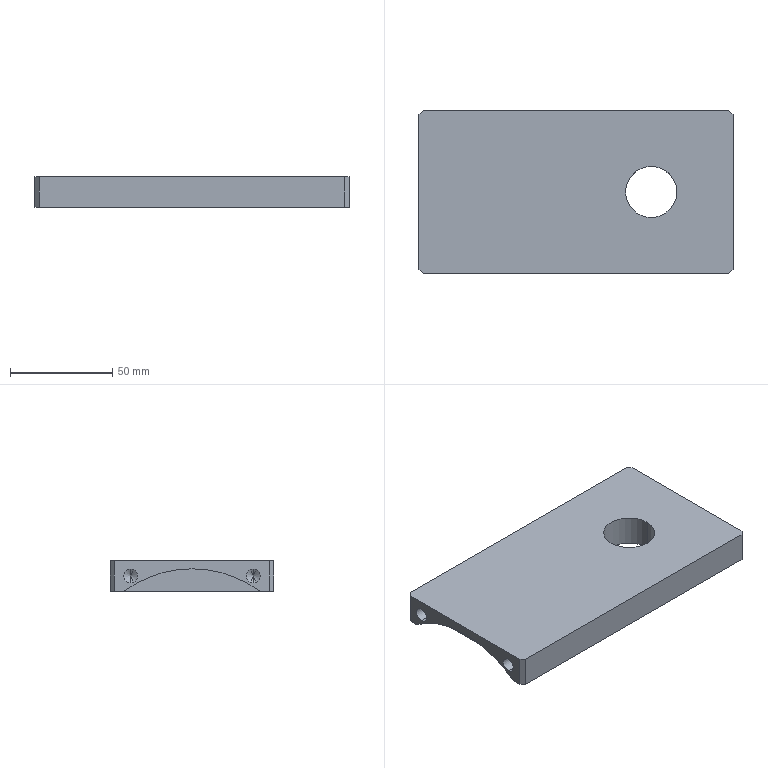Part | SolidWorks | features HoleWzd 2, Chamfer 1, Extrusion 1, ICE 1, MirrorPattern 1 | 1 solid | 31 faces | box 153.5 x 80 x 15 mm | volume 168755 mm3 | cylinder 12 | plane 11 | cone 8 | commonest cylinder face diameters 6.8 x8 25 x2 112 x2
STEP:
#1=CARTESIAN_POINT('',(-66.75,0.,3.5));
#2=VERTEX_POINT('',#1);
#3=CARTESIAN_POINT('',(-66.75,33.332,-7.5));
#4=VERTEX_POINT('',#3);
#5=CARTESIAN_POINT('',(-66.75,0.,-52.5));
#6=DIRECTION('',(-1.,0.,0.));
#7=DIRECTION('',(0.,0.,1.));
#8=AXIS2_PLACEMENT_3D('',#5,#6,#7);
#9=CIRCLE('',#8,56.);
#10=EDGE_CURVE('',#2,#4,#9,.T.);
#11=ORIENTED_EDGE('',*,*,#10,.F.);
#12=CARTESIAN_POINT('',(-76.75,0.,3.5));
#13=VERTEX_POINT('',#12);
#14=CARTESIAN_POINT('',(-66.75,0.,3.5));
#15=DIRECTION('',(-1.,0.,0.));
#16=VECTOR('',#15,1000.);
#17=LINE('',#14,#16);
#18=EDGE_CURVE('',#2,#13,#17,.T.);
#19=ORIENTED_EDGE('',*,*,#18,.T.);
#20=CARTESIAN_POINT('',(-76.75,33.332,-7.5));
#21=VERTEX_POINT('',#20);
#22=CARTESIAN_POINT('',(-76.75,0.,-52.5));
#23=DIRECTION('',(-1.,0.,0.));
#24=DIRECTION('',(0.,0.,1.));
#25=AXIS2_PLACEMENT_3D('',#22,#23,#24);
#26=CIRCLE('',#25,56.);
#27=EDGE_CURVE('',#13,#21,#26,.T.);
#28=ORIENTED_EDGE('',*,*,#27,.T.);
#29=CARTESIAN_POINT('',(-66.75,33.332,-7.5));
#30=DIRECTION('',(-1.,0.,0.));
#31=VECTOR('',#30,1000.);
#32=LINE('',#29,#31);
#33=EDGE_CURVE('',#4,#21,#32,.T.);
#34=ORIENTED_EDGE('',*,*,#33,.F.);
#35=EDGE_LOOP('',(#11,#19,#28,#34));
#36=FACE_OUTER_BOUND('',#35,.T.);
#37=CARTESIAN_POINT('',(-66.75,0.,-52.5));
#38=DIRECTION('',(-1.,0.,0.));
#39=DIRECTION('',(0.,0.,1.));
#40=AXIS2_PLACEMENT_3D('',#37,#38,#39);
#41=CYLINDRICAL_SURFACE('',#40,56.);
#42=ADVANCED_FACE('',(#36),#41,.F.);
#43=CARTESIAN_POINT('',(-57.,-30.,-3.4));
#44=VERTEX_POINT('',#43);
#45=CARTESIAN_POINT('',(-57.,-30.,3.4));
#46=VERTEX_POINT('',#45);
#47=CARTESIAN_POINT('',(-57.,-30.,0.));
#48=DIRECTION('',(-1.,0.,0.));
#49=DIRECTION('',(0.,0.,1.));
#50=AXIS2_PLACEMENT_3D('',#47,#48,#49);
#51=CIRCLE('',#50,3.4);
#52=EDGE_CURVE('',#44,#46,#51,.T.);
#53=ORIENTED_EDGE('',*,*,#52,.F.);
#54=CARTESIAN_POINT('',(-76.75,-30.,-3.4));
#55=VERTEX_POINT('',#54);
#56=CARTESIAN_POINT('',(-76.75,-30.,-3.4));
#57=DIRECTION('',(-1.,0.,0.));
#58=VECTOR('',#57,1000.);
#59=LINE('',#56,#58);
#60=EDGE_CURVE('',#44,#55,#59,.T.);
#61=ORIENTED_EDGE('',*,*,#60,.T.);
#62=CARTESIAN_POINT('',(-76.75,-30.,3.4));
#63=VERTEX_POINT('',#62);
#64=CARTESIAN_POINT('',(-76.75,-30.,0.));
#65=DIRECTION('',(-1.,0.,0.));
#66=DIRECTION('',(0.,0.,1.));
#67=AXIS2_PLACEMENT_3D('',#64,#65,#66);
#68=CIRCLE('',#67,3.4);
#69=EDGE_CURVE('',#55,#63,#68,.T.);
#70=ORIENTED_EDGE('',*,*,#69,.T.);
#71=CARTESIAN_POINT('',(-76.75,-30.,3.4));
#72=DIRECTION('',(-1.,0.,0.));
#73=VECTOR('',#72,1000.);
#74=LINE('',#71,#73);
#75=EDGE_CURVE('',#46,#63,#74,.T.);
#76=ORIENTED_EDGE('',*,*,#75,.F.);
#77=EDGE_LOOP('',(#53,#61,#70,#76));
#78=FACE_OUTER_BOUND('',#77,.T.);
#79=CARTESIAN_POINT('',(-76.75,-30.,0.));
#80=DIRECTION('',(-1.,0.,0.));
#81=DIRECTION('',(0.,0.,1.));
#82=AXIS2_PLACEMENT_3D('',#79,#80,#81);
#83=CYLINDRICAL_SURFACE('',#82,3.4);
#84=ADVANCED_FACE('',(#78),#83,.F.);
#85=CARTESIAN_POINT('',(-54.957,-30.,0.));
#86=VERTEX_POINT('',#85);
#87=CARTESIAN_POINT('',(-57.,-30.,3.4));
#88=DIRECTION('',(-0.515,0.,0.8572));
#89=VECTOR('',#88,1000.);
#90=LINE('',#87,#89);
#91=EDGE_CURVE('',#86,#46,#90,.T.);
#92=ORIENTED_EDGE('',*,*,#91,.F.);
#93=CARTESIAN_POINT('',(-57.,-30.,-3.4));
#94=DIRECTION('',(-0.515,0.,-0.8572));
#95=VECTOR('',#94,1000.);
#96=LINE('',#93,#95);
#97=EDGE_CURVE('',#86,#44,#96,.T.);
#98=ORIENTED_EDGE('',*,*,#97,.T.);
#99=ORIENTED_EDGE('',*,*,#52,.T.);
#100=EDGE_LOOP('',(#92,#98,#99));
#101=FACE_OUTER_BOUND('',#100,.T.);
#102=CARTESIAN_POINT('',(-57.,-30.,0.));
#103=DIRECTION('',(-1.,0.,0.));
#104=DIRECTION('',(0.,0.,1.));
#105=AXIS2_PLACEMENT_3D('',#102,#103,#104);
#106=CONICAL_SURFACE('',#105,3.4,1.03);
#107=ADVANCED_FACE('',(#101),#106,.F.);
#108=CARTESIAN_POINT('',(-57.,30.,-3.4));
#109=VERTEX_POINT('',#108);
#110=CARTESIAN_POINT('',(-57.,30.,3.4));
#111=VERTEX_POINT('',#110);
#112=CARTESIAN_POINT('',(-57.,30.,0.));
#113=DIRECTION('',(-1.,0.,0.));
#114=DIRECTION('',(0.,0.,1.));
#115=AXIS2_PLACEMENT_3D('',#112,#113,#114);
#116=CIRCLE('',#115,3.4);
#117=EDGE_CURVE('',#109,#111,#116,.T.);
#118=ORIENTED_EDGE('',*,*,#117,.F.);
#119=CARTESIAN_POINT('',(-76.75,30.,-3.4));
#120=VERTEX_POINT('',#119);
#121=CARTESIAN_POINT('',(-76.75,30.,-3.4));
#122=DIRECTION('',(-1.,0.,0.));
#123=VECTOR('',#122,1000.);
#124=LINE('',#121,#123);
#125=EDGE_CURVE('',#109,#120,#124,.T.);
#126=ORIENTED_EDGE('',*,*,#125,.T.);
#127=CARTESIAN_POINT('',(-76.75,30.,3.4));
#128=VERTEX_POINT('',#127);
#129=CARTESIAN_POINT('',(-76.75,30.,0.));
#130=DIRECTION('',(-1.,0.,0.));
#131=DIRECTION('',(0.,0.,1.));
#132=AXIS2_PLACEMENT_3D('',#129,#130,#131);
#133=CIRCLE('',#132,3.4);
#134=EDGE_CURVE('',#120,#128,#133,.T.);
#135=ORIENTED_EDGE('',*,*,#134,.T.);
#136=CARTESIAN_POINT('',(-76.75,30.,3.4));
#137=DIRECTION('',(-1.,0.,0.));
#138=VECTOR('',#137,1000.);
#139=LINE('',#136,#138);
#140=EDGE_CURVE('',#111,#128,#139,.T.);
#141=ORIENTED_EDGE('',*,*,#140,.F.);
#142=EDGE_LOOP('',(#118,#126,#135,#141));
#143=FACE_OUTER_BOUND('',#142,.T.);
#144=CARTESIAN_POINT('',(-76.75,30.,0.));
#145=DIRECTION('',(-1.,0.,0.));
#146=DIRECTION('',(0.,0.,1.));
#147=AXIS2_PLACEMENT_3D('',#144,#145,#146);
#148=CYLINDRICAL_SURFACE('',#147,3.4);
#149=ADVANCED_FACE('',(#143),#148,.F.);
#150=CARTESIAN_POINT('',(-54.957,30.,0.));
#151=VERTEX_POINT('',#150);
#152=CARTESIAN_POINT('',(-57.,30.,3.4));
#153=DIRECTION('',(-0.515,0.,0.8572));
#154=VECTOR('',#153,1000.);
#155=LINE('',#152,#154);
#156=EDGE_CURVE('',#151,#111,#155,.T.);
#157=ORIENTED_EDGE('',*,*,#156,.F.);
#158=CARTESIAN_POINT('',(-57.,30.,-3.4));
#159=DIRECTION('',(-0.515,0.,-0.8572));
#160=VECTOR('',#159,1000.);
#161=LINE('',#158,#160);
#162=EDGE_CURVE('',#151,#109,#161,.T.);
#163=ORIENTED_EDGE('',*,*,#162,.T.);
#164=ORIENTED_EDGE('',*,*,#117,.T.);
#165=EDGE_LOOP('',(#157,#163,#164));
#166=FACE_OUTER_BOUND('',#165,.T.);
#167=CARTESIAN_POINT('',(-57.,30.,0.));
#168=DIRECTION('',(-1.,0.,0.));
#169=DIRECTION('',(0.,0.,1.));
#170=AXIS2_PLACEMENT_3D('',#167,#168,#169);
#171=CONICAL_SURFACE('',#170,3.4,1.03);
#172=ADVANCED_FACE('',(#166),#171,.F.);
#173=CARTESIAN_POINT('',(57.,-30.,3.4));
#174=VERTEX_POINT('',#173);
#175=CARTESIAN_POINT('',(57.,-30.,-3.4));
#176=VERTEX_POINT('',#175);
#177=CARTESIAN_POINT('',(57.,-30.,0.));
#178=DIRECTION('',(1.,0.,0.));
#179=DIRECTION('',(0.,0.,-1.));
#180=AXIS2_PLACEMENT_3D('',#177,#178,#179);
#181=CIRCLE('',#180,3.4);
#182=EDGE_CURVE('',#174,#176,#181,.T.);
#183=ORIENTED_EDGE('',*,*,#182,.F.);
#184=CARTESIAN_POINT('',(76.75,-30.,3.4));
#185=VERTEX_POINT('',#184);
#186=CARTESIAN_POINT('',(76.75,-30.,3.4));
#187=DIRECTION('',(1.,0.,0.));
#188=VECTOR('',#187,1000.);
#189=LINE('',#186,#188);
#190=EDGE_CURVE('',#174,#185,#189,.T.);
#191=ORIENTED_EDGE('',*,*,#190,.T.);
#192=CARTESIAN_POINT('',(76.75,-30.,-3.4));
#193=VERTEX_POINT('',#192);
#194=CARTESIAN_POINT('',(76.75,-30.,0.));
#195=DIRECTION('',(1.,0.,0.));
#196=DIRECTION('',(0.,0.,-1.));
#197=AXIS2_PLACEMENT_3D('',#194,#195,#196);
#198=CIRCLE('',#197,3.4);
#199=EDGE_CURVE('',#185,#193,#198,.T.);
#200=ORIENTED_EDGE('',*,*,#199,.T.);
#201=CARTESIAN_POINT('',(76.75,-30.,-3.4));
#202=DIRECTION('',(1.,0.,0.));
#203=VECTOR('',#202,1000.);
#204=LINE('',#201,#203);
#205=EDGE_CURVE('',#176,#193,#204,.T.);
#206=ORIENTED_EDGE('',*,*,#205,.F.);
#207=EDGE_LOOP('',(#183,#191,#200,#206));
#208=FACE_OUTER_BOUND('',#207,.T.);
#209=CARTESIAN_POINT('',(76.75,-30.,0.));
#210=DIRECTION('',(1.,0.,0.));
#211=DIRECTION('',(0.,0.,-1.));
#212=AXIS2_PLACEMENT_3D('',#209,#210,#211);
#213=CYLINDRICAL_SURFACE('',#212,3.4);
#214=ADVANCED_FACE('',(#208),#213,.F.);
#215=CARTESIAN_POINT('',(54.957,-30.,0.));
#216=VERTEX_POINT('',#215);
#217=CARTESIAN_POINT('',(57.,-30.,-3.4));
#218=DIRECTION('',(0.515,0.,-0.8572));
#219=VECTOR('',#218,1000.);
#220=LINE('',#217,#219);
#221=EDGE_CURVE('',#216,#176,#220,.T.);
#222=ORIENTED_EDGE('',*,*,#221,.F.);
#223=CARTESIAN_POINT('',(57.,-30.,3.4));
#224=DIRECTION('',(0.515,0.,0.8572));
#225=VECTOR('',#224,1000.);
#226=LINE('',#223,#225);
#227=EDGE_CURVE('',#216,#174,#226,.T.);
#228=ORIENTED_EDGE('',*,*,#227,.T.);
#229=ORIENTED_EDGE('',*,*,#182,.T.);
#230=EDGE_LOOP('',(#222,#228,#229));
#231=FACE_OUTER_BOUND('',#230,.T.);
#232=CARTESIAN_POINT('',(57.,-30.,0.));
#233=DIRECTION('',(1.,0.,0.));
#234=DIRECTION('',(0.,0.,-1.));
#235=AXIS2_PLACEMENT_3D('',#232,#233,#234);
#236=CONICAL_SURFACE('',#235,3.4,1.03);
#237=ADVANCED_FACE('',(#231),#236,.F.);
#238=CARTESIAN_POINT('',(57.,30.,3.4));
#239=VERTEX_POINT('',#238);
#240=CARTESIAN_POINT('',(57.,30.,-3.4));
#241=VERTEX_POINT('',#240);
#242=CARTESIAN_POINT('',(57.,30.,0.));
#243=DIRECTION('',(1.,0.,0.));
#244=DIRECTION('',(0.,0.,-1.));
#245=AXIS2_PLACEMENT_3D('',#242,#243,#244);
#246=CIRCLE('',#245,3.4);
#247=EDGE_CURVE('',#239,#241,#246,.T.);
#248=ORIENTED_EDGE('',*,*,#247,.F.);
#249=CARTESIAN_POINT('',(76.75,30.,3.4));
#250=VERTEX_POINT('',#249);
#251=CARTESIAN_POINT('',(76.75,30.,3.4));
#252=DIRECTION('',(1.,0.,0.));
#253=VECTOR('',#252,1000.);
#254=LINE('',#251,#253);
#255=EDGE_CURVE('',#239,#250,#254,.T.);
#256=ORIENTED_EDGE('',*,*,#255,.T.);
#257=CARTESIAN_POINT('',(76.75,30.,-3.4));
#258=VERTEX_POINT('',#257);
#259=CARTESIAN_POINT('',(76.75,30.,0.));
#260=DIRECTION('',(1.,0.,0.));
#261=DIRECTION('',(0.,0.,-1.));
#262=AXIS2_PLACEMENT_3D('',#259,#260,#261);
#263=CIRCLE('',#262,3.4);
#264=EDGE_CURVE('',#250,#258,#263,.T.);
#265=ORIENTED_EDGE('',*,*,#264,.T.);
#266=CARTESIAN_POINT('',(76.75,30.,-3.4));
#267=DIRECTION('',(1.,0.,0.));
#268=VECTOR('',#267,1000.);
#269=LINE('',#266,#268);
#270=EDGE_CURVE('',#241,#258,#269,.T.);
#271=ORIENTED_EDGE('',*,*,#270,.F.);
#272=EDGE_LOOP('',(#248,#256,#265,#271));
#273=FACE_OUTER_BOUND('',#272,.T.);
#274=CARTESIAN_POINT('',(76.75,30.,0.));
#275=DIRECTION('',(1.,0.,0.));
#276=DIRECTION('',(0.,0.,-1.));
#277=AXIS2_PLACEMENT_3D('',#274,#275,#276);
#278=CYLINDRICAL_SURFACE('',#277,3.4);
#279=ADVANCED_FACE('',(#273),#278,.F.);
#280=CARTESIAN_POINT('',(54.957,30.,0.));
#281=VERTEX_POINT('',#280);
#282=CARTESIAN_POINT('',(57.,30.,-3.4));
#283=DIRECTION('',(0.515,0.,-0.8572));
#284=VECTOR('',#283,1000.);
#285=LINE('',#282,#284);
#286=EDGE_CURVE('',#281,#241,#285,.T.);
#287=ORIENTED_EDGE('',*,*,#286,.F.);
#288=CARTESIAN_POINT('',(57.,30.,3.4));
#289=DIRECTION('',(0.515,0.,0.8572));
#290=VECTOR('',#289,1000.);
#291=LINE('',#288,#290);
#292=EDGE_CURVE('',#281,#239,#291,.T.);
#293=ORIENTED_EDGE('',*,*,#292,.T.);
#294=ORIENTED_EDGE('',*,*,#247,.T.);
#295=EDGE_LOOP('',(#287,#293,#294));
#296=FACE_OUTER_BOUND('',#295,.T.);
#297=CARTESIAN_POINT('',(57.,30.,0.));
#298=DIRECTION('',(1.,0.,0.));
#299=DIRECTION('',(0.,0.,-1.));
#300=AXIS2_PLACEMENT_3D('',#297,#298,#299);
#301=CONICAL_SURFACE('',#300,3.4,1.03);
#302=ADVANCED_FACE('',(#296),#301,.F.);
#303=CARTESIAN_POINT('',(24.25,0.,-7.5));
#304=VERTEX_POINT('',#303);
#305=CARTESIAN_POINT('',(49.25,0.,-7.5));
#306=VERTEX_POINT('',#305);
#307=CARTESIAN_POINT('',(36.75,0.,-7.5));
#308=DIRECTION('',(0.,0.,1.));
#309=DIRECTION('',(1.,0.,0.));
#310=AXIS2_PLACEMENT_3D('',#307,#308,#309);
#311=CIRCLE('',#310,12.5);
#312=EDGE_CURVE('',#304,#306,#311,.T.);
#313=ORIENTED_EDGE('',*,*,#312,.F.);
#314=CARTESIAN_POINT('',(24.25,0.,7.5));
#315=VERTEX_POINT('',#314);
#316=CARTESIAN_POINT('',(24.25,0.,7.5));
#317=DIRECTION('',(0.,0.,1.));
#318=VECTOR('',#317,1000.);
#319=LINE('',#316,#318);
#320=EDGE_CURVE('',#304,#315,#319,.T.);
#321=ORIENTED_EDGE('',*,*,#320,.T.);
#322=CARTESIAN_POINT('',(49.25,0.,7.5));
#323=VERTEX_POINT('',#322);
#324=CARTESIAN_POINT('',(36.75,0.,7.5));
#325=DIRECTION('',(0.,0.,1.));
#326=DIRECTION('',(1.,0.,0.));
#327=AXIS2_PLACEMENT_3D('',#324,#325,#326);
#328=CIRCLE('',#327,12.5);
#329=EDGE_CURVE('',#315,#323,#328,.T.);
#330=ORIENTED_EDGE('',*,*,#329,.T.);
#331=CARTESIAN_POINT('',(49.25,0.,7.5));
#332=DIRECTION('',(0.,0.,1.));
#333=VECTOR('',#332,1000.);
#334=LINE('',#331,#333);
#335=EDGE_CURVE('',#306,#323,#334,.T.);
#336=ORIENTED_EDGE('',*,*,#335,.F.);
#337=EDGE_LOOP('',(#313,#321,#330,#336));
#338=FACE_OUTER_BOUND('',#337,.T.);
#339=CARTESIAN_POINT('',(36.75,0.,7.5));
#340=DIRECTION('',(0.,0.,1.));
#341=DIRECTION('',(1.,0.,0.));
#342=AXIS2_PLACEMENT_3D('',#339,#340,#341);
#343=CYLINDRICAL_SURFACE('',#342,12.5);
#344=ADVANCED_FACE('',(#338),#343,.F.);
#345=CARTESIAN_POINT('',(76.75,-30.,0.));
#346=DIRECTION('',(1.,0.,0.));
#347=DIRECTION('',(0.,0.,-1.));
#348=AXIS2_PLACEMENT_3D('',#345,#346,#347);
#349=CIRCLE('',#348,3.4);
#350=EDGE_CURVE('',#193,#185,#349,.T.);
#351=ORIENTED_EDGE('',*,*,#350,.F.);
#352=ORIENTED_EDGE('',*,*,#199,.F.);
#353=EDGE_LOOP('',(#351,#352));
#354=FACE_BOUND('',#353,.T.);
#355=CARTESIAN_POINT('',(76.75,30.,0.));
#356=DIRECTION('',(1.,0.,0.));
#357=DIRECTION('',(0.,0.,-1.));
#358=AXIS2_PLACEMENT_3D('',#355,#356,#357);
#359=CIRCLE('',#358,3.4);
#360=EDGE_CURVE('',#258,#250,#359,.T.);
#361=ORIENTED_EDGE('',*,*,#360,.F.);
#362=ORIENTED_EDGE('',*,*,#264,.F.);
#363=EDGE_LOOP('',(#361,#362));
#364=FACE_BOUND('',#363,.T.);
#365=CARTESIAN_POINT('',(76.75,-38.,-7.5));
#366=VERTEX_POINT('',#365);
#367=CARTESIAN_POINT('',(76.75,38.,-7.5));
#368=VERTEX_POINT('',#367);
#369=CARTESIAN_POINT('',(76.75,40.,-7.5));
#370=DIRECTION('',(0.,1.,0.));
#371=VECTOR('',#370,1000.);
#372=LINE('',#369,#371);
#373=EDGE_CURVE('',#366,#368,#372,.T.);
#374=ORIENTED_EDGE('',*,*,#373,.T.);
#375=CARTESIAN_POINT('',(76.75,38.,7.5));
#376=VERTEX_POINT('',#375);
#377=CARTESIAN_POINT('',(76.75,38.,7.5));
#378=DIRECTION('',(0.,0.,1.));
#379=VECTOR('',#378,1000.);
#380=LINE('',#377,#379);
#381=EDGE_CURVE('',#368,#376,#380,.T.);
#382=ORIENTED_EDGE('',*,*,#381,.T.);
#383=CARTESIAN_POINT('',(76.75,-38.,7.5));
#384=VERTEX_POINT('',#383);
#385=CARTESIAN_POINT('',(76.75,40.,7.5));
#386=DIRECTION('',(0.,1.,0.));
#387=VECTOR('',#386,1000.);
#388=LINE('',#385,#387);
#389=EDGE_CURVE('',#384,#376,#388,.T.);
#390=ORIENTED_EDGE('',*,*,#389,.F.);
#391=CARTESIAN_POINT('',(76.75,-38.,7.5));
#392=DIRECTION('',(0.,0.,-1.));
#393=VECTOR('',#392,1000.);
#394=LINE('',#391,#393);
#395=EDGE_CURVE('',#384,#366,#394,.T.);
#396=ORIENTED_EDGE('',*,*,#395,.T.);
#397=EDGE_LOOP('',(#374,#382,#390,#396));
#398=FACE_OUTER_BOUND('',#397,.T.);
#399=CARTESIAN_POINT('',(76.75,40.,7.5));
#400=DIRECTION('',(-1.,0.,0.));
#401=DIRECTION('',(0.,-1.,0.));
#402=AXIS2_PLACEMENT_3D('',#399,#400,#401);
#403=PLANE('',#402);
#404=ADVANCED_FACE('',(#354,#364,#398),#403,.F.);
#405=CARTESIAN_POINT('',(74.75,40.,7.5));
#406=VERTEX_POINT('',#405);
#407=CARTESIAN_POINT('',(-74.75,40.,7.5));
#408=VERTEX_POINT('',#407);
#409=CARTESIAN_POINT('',(-76.75,40.,7.5));
#410=DIRECTION('',(-1.,0.,0.));
#411=VECTOR('',#410,1000.);
#412=LINE('',#409,#411);
#413=EDGE_CURVE('',#406,#408,#412,.T.);
#414=ORIENTED_EDGE('',*,*,#413,.F.);
#415=CARTESIAN_POINT('',(74.75,40.,-7.5));
#416=VERTEX_POINT('',#415);
#417=CARTESIAN_POINT('',(74.75,40.,7.5));
#418=DIRECTION('',(0.,0.,-1.));
#419=VECTOR('',#418,1000.);
#420=LINE('',#417,#419);
#421=EDGE_CURVE('',#406,#416,#420,.T.);
#422=ORIENTED_EDGE('',*,*,#421,.T.);
#423=CARTESIAN_POINT('',(-74.75,40.,-7.5));
#424=VERTEX_POINT('',#423);
#425=CARTESIAN_POINT('',(-76.75,40.,-7.5));
#426=DIRECTION('',(-1.,0.,0.));
#427=VECTOR('',#426,1000.);
#428=LINE('',#425,#427);
#429=EDGE_CURVE('',#416,#424,#428,.T.);
#430=ORIENTED_EDGE('',*,*,#429,.T.);
#431=CARTESIAN_POINT('',(-74.75,40.,7.5));
#432=DIRECTION('',(0.,0.,1.));
#433=VECTOR('',#432,1000.);
#434=LINE('',#431,#433);
#435=EDGE_CURVE('',#424,#408,#434,.T.);
#436=ORIENTED_EDGE('',*,*,#435,.T.);
#437=EDGE_LOOP('',(#414,#422,#430,#436));
#438=FACE_OUTER_BOUND('',#437,.T.);
#439=CARTESIAN_POINT('',(-76.75,40.,7.5));
#440=DIRECTION('',(0.,-1.,0.));
#441=DIRECTION('',(0.,0.,-1.));
#442=AXIS2_PLACEMENT_3D('',#439,#440,#441);
#443=PLANE('',#442);
#444=ADVANCED_FACE('',(#438),#443,.F.);
#445=CARTESIAN_POINT('',(-76.75,-30.,0.));
#446=DIRECTION('',(-1.,0.,0.));
#447=DIRECTION('',(0.,0.,1.));
#448=AXIS2_PLACEMENT_3D('',#445,#446,#447);
#449=CIRCLE('',#448,3.4);
#450=EDGE_CURVE('',#63,#55,#449,.T.);
#451=ORIENTED_EDGE('',*,*,#450,.F.);
#452=ORIENTED_EDGE('',*,*,#69,.F.);
#453=EDGE_LOOP('',(#451,#452));
#454=FACE_BOUND('',#453,.T.);
#455=CARTESIAN_POINT('',(-76.75,30.,0.));
#456=DIRECTION('',(-1.,0.,0.));
#457=DIRECTION('',(0.,0.,1.));
#458=AXIS2_PLACEMENT_3D('',#455,#456,#457);
#459=CIRCLE('',#458,3.4);
#460=EDGE_CURVE('',#128,#120,#459,.T.);
#461=ORIENTED_EDGE('',*,*,#460,.F.);
#462=ORIENTED_EDGE('',*,*,#134,.F.);
#463=EDGE_LOOP('',(#461,#462));
#464=FACE_BOUND('',#463,.T.);
#465=CARTESIAN_POINT('',(-76.75,-33.332,-7.5));
#466=VERTEX_POINT('',#465);
#467=CARTESIAN_POINT('',(-76.75,-38.,-7.5));
#468=VERTEX_POINT('',#467);
#469=CARTESIAN_POINT('',(-76.75,40.,-7.5));
#470=DIRECTION('',(0.,-1.,0.));
#471=VECTOR('',#470,1000.);
#472=LINE('',#469,#471);
#473=EDGE_CURVE('',#466,#468,#472,.T.);
#474=ORIENTED_EDGE('',*,*,#473,.T.);
#475=CARTESIAN_POINT('',(-76.75,-38.,7.5));
#476=VERTEX_POINT('',#475);
#477=CARTESIAN_POINT('',(-76.75,-38.,7.5));
#478=DIRECTION('',(0.,0.,1.));
#479=VECTOR('',#478,1000.);
#480=LINE('',#477,#479);
#481=EDGE_CURVE('',#468,#476,#480,.T.);
#482=ORIENTED_EDGE('',*,*,#481,.T.);
#483=CARTESIAN_POINT('',(-76.75,38.,7.5));
#484=VERTEX_POINT('',#483);
#485=CARTESIAN_POINT('',(-76.75,40.,7.5));
#486=DIRECTION('',(0.,-1.,0.));
#487=VECTOR('',#486,1000.);
#488=LINE('',#485,#487);
#489=EDGE_CURVE('',#484,#476,#488,.T.);
#490=ORIENTED_EDGE('',*,*,#489,.F.);
#491=CARTESIAN_POINT('',(-76.75,38.,-7.5));
#492=VERTEX_POINT('',#491);
#493=CARTESIAN_POINT('',(-76.75,38.,7.5));
#494=DIRECTION('',(0.,0.,-1.));
#495=VECTOR('',#494,1000.);
#496=LINE('',#493,#495);
#497=EDGE_CURVE('',#484,#492,#496,.T.);
#498=ORIENTED_EDGE('',*,*,#497,.T.);
#499=CARTESIAN_POINT('',(-76.75,40.,-7.5));
#500=DIRECTION('',(0.,-1.,0.));
#501=VECTOR('',#500,1000.);
#502=LINE('',#499,#501);
#503=EDGE_CURVE('',#492,#21,#502,.T.);
#504=ORIENTED_EDGE('',*,*,#503,.T.);
#505=ORIENTED_EDGE('',*,*,#27,.F.);
#506=CARTESIAN_POINT('',(-76.75,0.,-52.5));
#507=DIRECTION('',(-1.,0.,0.));
#508=DIRECTION('',(0.,0.,1.));
#509=AXIS2_PLACEMENT_3D('',#506,#507,#508);
#510=CIRCLE('',#509,56.);
#511=EDGE_CURVE('',#466,#13,#510,.T.);
#512=ORIENTED_EDGE('',*,*,#511,.F.);
#513=EDGE_LOOP('',(#474,#482,#490,#498,#504,#505,#512));
#514=FACE_OUTER_BOUND('',#513,.T.);
#515=CARTESIAN_POINT('',(-76.75,40.,7.5));
#516=DIRECTION('',(1.,0.,0.));
#517=DIRECTION('',(0.,0.,-1.));
#518=AXIS2_PLACEMENT_3D('',#515,#516,#517);
#519=PLANE('',#518);
#520=ADVANCED_FACE('',(#454,#464,#514),#519,.F.);
#521=CARTESIAN_POINT('',(-74.75,-40.,-7.5));
#522=VERTEX_POINT('',#521);
#523=CARTESIAN_POINT('',(74.75,-40.,-7.5));
#524=VERTEX_POINT('',#523);
#525=CARTESIAN_POINT('',(-76.75,-40.,-7.5));
#526=DIRECTION('',(1.,0.,0.));
#527=VECTOR('',#526,1000.);
#528=LINE('',#525,#527);
#529=EDGE_CURVE('',#522,#524,#528,.T.);
#530=ORIENTED_EDGE('',*,*,#529,.T.);
#531=CARTESIAN_POINT('',(74.75,-40.,7.5));
#532=VERTEX_POINT('',#531);
#533=CARTESIAN_POINT('',(74.75,-40.,7.5));
#534=DIRECTION('',(0.,0.,1.));
#535=VECTOR('',#534,1000.);
#536=LINE('',#533,#535);
#537=EDGE_CURVE('',#524,#532,#536,.T.);
#538=ORIENTED_EDGE('',*,*,#537,.T.);
#539=CARTESIAN_POINT('',(-74.75,-40.,7.5));
#540=VERTEX_POINT('',#539);
#541=CARTESIAN_POINT('',(-76.75,-40.,7.5));
#542=DIRECTION('',(1.,0.,0.));
#543=VECTOR('',#542,1000.);
#544=LINE('',#541,#543);
#545=EDGE_CURVE('',#540,#532,#544,.T.);
#546=ORIENTED_EDGE('',*,*,#545,.F.);
#547=CARTESIAN_POINT('',(-74.75,-40.,7.5));
#548=DIRECTION('',(0.,0.,-1.));
#549=VECTOR('',#548,1000.);
#550=LINE('',#547,#549);
#551=EDGE_CURVE('',#540,#522,#550,.T.);
#552=ORIENTED_EDGE('',*,*,#551,.T.);
#553=EDGE_LOOP('',(#530,#538,#546,#552));
#554=FACE_OUTER_BOUND('',#553,.T.);
#555=CARTESIAN_POINT('',(-76.75,-40.,7.5));
#556=DIRECTION('',(0.,1.,0.));
#557=DIRECTION('',(0.,0.,1.));
#558=AXIS2_PLACEMENT_3D('',#555,#556,#557);
#559=PLANE('',#558);
#560=ADVANCED_FACE('',(#554),#559,.F.);
#561=CARTESIAN_POINT('',(36.75,0.,7.5));
#562=DIRECTION('',(0.,0.,1.));
#563=DIRECTION('',(1.,0.,0.));
#564=AXIS2_PLACEMENT_3D('',#561,#562,#563);
#565=CIRCLE('',#564,12.5);
#566=EDGE_CURVE('',#323,#315,#565,.T.);
#567=ORIENTED_EDGE('',*,*,#566,.F.);
#568=ORIENTED_EDGE('',*,*,#329,.F.);
#569=EDGE_LOOP('',(#567,#568));
#570=FACE_BOUND('',#569,.T.);
#571=ORIENTED_EDGE('',*,*,#389,.T.);
#572=CARTESIAN_POINT('',(57.375,57.375,7.5));
#573=DIRECTION('',(-0.7071,0.7071,0.));
#574=VECTOR('',#573,1000.);
#575=LINE('',#572,#574);
#576=EDGE_CURVE('',#376,#406,#575,.T.);
#577=ORIENTED_EDGE('',*,*,#576,.T.);
#578=ORIENTED_EDGE('',*,*,#413,.T.);
#579=CARTESIAN_POINT('',(-57.375,57.375,7.5));
#580=DIRECTION('',(-0.7071,-0.7071,0.));
#581=VECTOR('',#580,1000.);
#582=LINE('',#579,#581);
#583=EDGE_CURVE('',#408,#484,#582,.T.);
#584=ORIENTED_EDGE('',*,*,#583,.T.);
#585=ORIENTED_EDGE('',*,*,#489,.T.);
#586=CARTESIAN_POINT('',(-57.375,-57.375,7.5));
#587=DIRECTION('',(0.7071,-0.7071,0.));
#588=VECTOR('',#587,1000.);
#589=LINE('',#586,#588);
#590=EDGE_CURVE('',#476,#540,#589,.T.);
#591=ORIENTED_EDGE('',*,*,#590,.T.);
#592=ORIENTED_EDGE('',*,*,#545,.T.);
#593=CARTESIAN_POINT('',(57.375,-57.375,7.5));
#594=DIRECTION('',(0.7071,0.7071,0.));
#595=VECTOR('',#594,1000.);
#596=LINE('',#593,#595);
#597=EDGE_CURVE('',#532,#384,#596,.T.);
#598=ORIENTED_EDGE('',*,*,#597,.T.);
#599=EDGE_LOOP('',(#571,#577,#578,#584,#585,#591,#592,#598));
#600=FACE_OUTER_BOUND('',#599,.T.);
#601=CARTESIAN_POINT('',(0.,0.,7.5));
#602=DIRECTION('',(0.,0.,1.));
#603=DIRECTION('',(1.,0.,0.));
#604=AXIS2_PLACEMENT_3D('',#601,#602,#603);
#605=PLANE('',#604);
#606=ADVANCED_FACE('',(#570,#600),#605,.T.);
#607=CARTESIAN_POINT('',(36.75,0.,-7.5));
#608=DIRECTION('',(0.,0.,1.));
#609=DIRECTION('',(1.,0.,0.));
#610=AXIS2_PLACEMENT_3D('',#607,#608,#609);
#611=CIRCLE('',#610,12.5);
#612=EDGE_CURVE('',#306,#304,#611,.T.);
#613=ORIENTED_EDGE('',*,*,#612,.T.);
#614=ORIENTED_EDGE('',*,*,#312,.T.);
#615=EDGE_LOOP('',(#613,#614));
#616=FACE_BOUND('',#615,.T.);
#617=ORIENTED_EDGE('',*,*,#429,.F.);
#618=CARTESIAN_POINT('',(74.75,40.,-7.5));
#619=DIRECTION('',(0.7071,-0.7071,0.));
#620=VECTOR('',#619,1000.);
#621=LINE('',#618,#620);
#622=EDGE_CURVE('',#416,#368,#621,.T.);
#623=ORIENTED_EDGE('',*,*,#622,.T.);
#624=ORIENTED_EDGE('',*,*,#373,.F.);
#625=CARTESIAN_POINT('',(76.75,-38.,-7.5));
#626=DIRECTION('',(-0.7071,-0.7071,0.));
#627=VECTOR('',#626,1000.);
#628=LINE('',#625,#627);
#629=EDGE_CURVE('',#366,#524,#628,.T.);
#630=ORIENTED_EDGE('',*,*,#629,.T.);
#631=ORIENTED_EDGE('',*,*,#529,.F.);
#632=CARTESIAN_POINT('',(-74.75,-40.,-7.5));
#633=DIRECTION('',(-0.7071,0.7071,0.));
#634=VECTOR('',#633,1000.);
#635=LINE('',#632,#634);
#636=EDGE_CURVE('',#522,#468,#635,.T.);
#637=ORIENTED_EDGE('',*,*,#636,.T.);
#638=ORIENTED_EDGE('',*,*,#473,.F.);
#639=CARTESIAN_POINT('',(-66.75,-33.332,-7.5));
#640=VERTEX_POINT('',#639);
#641=CARTESIAN_POINT('',(-66.75,-33.332,-7.5));
#642=DIRECTION('',(1.,0.,0.));
#643=VECTOR('',#642,1000.);
#644=LINE('',#641,#643);
#645=EDGE_CURVE('',#466,#640,#644,.T.);
#646=ORIENTED_EDGE('',*,*,#645,.T.);
#647=CARTESIAN_POINT('',(-66.75,0.,-7.5));
#648=DIRECTION('',(0.,-1.,0.));
#649=VECTOR('',#648,1000.);
#650=LINE('',#647,#649);
#651=EDGE_CURVE('',#4,#640,#650,.T.);
#652=ORIENTED_EDGE('',*,*,#651,.F.);
#653=ORIENTED_EDGE('',*,*,#33,.T.);
#654=ORIENTED_EDGE('',*,*,#503,.F.);
#655=CARTESIAN_POINT('',(-76.75,38.,-7.5));
#656=DIRECTION('',(0.7071,0.7071,0.));
#657=VECTOR('',#656,1000.);
#658=LINE('',#655,#657);
#659=EDGE_CURVE('',#492,#424,#658,.T.);
#660=ORIENTED_EDGE('',*,*,#659,.T.);
#661=EDGE_LOOP('',(#617,#623,#624,#630,#631,#637,#638,#646,#652,#653,#654,#660));
#662=FACE_OUTER_BOUND('',#661,.T.);
#663=CARTESIAN_POINT('',(0.,0.,-7.5));
#664=DIRECTION('',(0.,0.,1.));
#665=DIRECTION('',(1.,0.,0.));
#666=AXIS2_PLACEMENT_3D('',#663,#664,#665);
#667=PLANE('',#666);
#668=ADVANCED_FACE('',(#616,#662),#667,.F.);
#669=ORIENTED_EDGE('',*,*,#320,.F.);
#670=ORIENTED_EDGE('',*,*,#612,.F.);
#671=ORIENTED_EDGE('',*,*,#335,.T.);
#672=ORIENTED_EDGE('',*,*,#566,.T.);
#673=EDGE_LOOP('',(#669,#670,#671,#672));
#674=FACE_OUTER_BOUND('',#673,.T.);
#675=CARTESIAN_POINT('',(36.75,0.,7.5));
#676=DIRECTION('',(0.,0.,1.));
#677=DIRECTION('',(1.,0.,0.));
#678=AXIS2_PLACEMENT_3D('',#675,#676,#677);
#679=CYLINDRICAL_SURFACE('',#678,12.5);
#680=ADVANCED_FACE('',(#674),#679,.F.);
#681=ORIENTED_EDGE('',*,*,#292,.F.);
#682=ORIENTED_EDGE('',*,*,#286,.T.);
#683=CARTESIAN_POINT('',(57.,30.,0.));
#684=DIRECTION('',(1.,0.,0.));
#685=DIRECTION('',(0.,0.,-1.));
#686=AXIS2_PLACEMENT_3D('',#683,#684,#685);
#687=CIRCLE('',#686,3.4);
#688=EDGE_CURVE('',#241,#239,#687,.T.);
#689=ORIENTED_EDGE('',*,*,#688,.T.);
#690=EDGE_LOOP('',(#681,#682,#689));
#691=FACE_OUTER_BOUND('',#690,.T.);
#692=CARTESIAN_POINT('',(57.,30.,0.));
#693=DIRECTION('',(1.,0.,0.));
#694=DIRECTION('',(0.,0.,-1.));
#695=AXIS2_PLACEMENT_3D('',#692,#693,#694);
#696=CONICAL_SURFACE('',#695,3.4,1.03);
#697=ADVANCED_FACE('',(#691),#696,.F.);
#698=ORIENTED_EDGE('',*,*,#255,.F.);
#699=ORIENTED_EDGE('',*,*,#688,.F.);
#700=ORIENTED_EDGE('',*,*,#270,.T.);
#701=ORIENTED_EDGE('',*,*,#360,.T.);
#702=EDGE_LOOP('',(#698,#699,#700,#701));
#703=FACE_OUTER_BOUND('',#702,.T.);
#704=CARTESIAN_POINT('',(76.75,30.,0.));
#705=DIRECTION('',(1.,0.,0.));
#706=DIRECTION('',(0.,0.,-1.));
#707=AXIS2_PLACEMENT_3D('',#704,#705,#706);
#708=CYLINDRICAL_SURFACE('',#707,3.4);
#709=ADVANCED_FACE('',(#703),#708,.F.);
#710=ORIENTED_EDGE('',*,*,#227,.F.);
#711=ORIENTED_EDGE('',*,*,#221,.T.);
#712=CARTESIAN_POINT('',(57.,-30.,0.));
#713=DIRECTION('',(1.,0.,0.));
#714=DIRECTION('',(0.,0.,-1.));
#715=AXIS2_PLACEMENT_3D('',#712,#713,#714);
#716=CIRCLE('',#715,3.4);
#717=EDGE_CURVE('',#176,#174,#716,.T.);
#718=ORIENTED_EDGE('',*,*,#717,.T.);
#719=EDGE_LOOP('',(#710,#711,#718));
#720=FACE_OUTER_BOUND('',#719,.T.);
#721=CARTESIAN_POINT('',(57.,-30.,0.));
#722=DIRECTION('',(1.,0.,0.));
#723=DIRECTION('',(0.,0.,-1.));
#724=AXIS2_PLACEMENT_3D('',#721,#722,#723);
#725=CONICAL_SURFACE('',#724,3.4,1.03);
#726=ADVANCED_FACE('',(#720),#725,.F.);
#727=ORIENTED_EDGE('',*,*,#190,.F.);
#728=ORIENTED_EDGE('',*,*,#717,.F.);
#729=ORIENTED_EDGE('',*,*,#205,.T.);
#730=ORIENTED_EDGE('',*,*,#350,.T.);
#731=EDGE_LOOP('',(#727,#728,#729,#730));
#732=FACE_OUTER_BOUND('',#731,.T.);
#733=CARTESIAN_POINT('',(76.75,-30.,0.));
#734=DIRECTION('',(1.,0.,0.));
#735=DIRECTION('',(0.,0.,-1.));
#736=AXIS2_PLACEMENT_3D('',#733,#734,#735);
#737=CYLINDRICAL_SURFACE('',#736,3.4);
#738=ADVANCED_FACE('',(#732),#737,.F.);
#739=ORIENTED_EDGE('',*,*,#162,.F.);
#740=ORIENTED_EDGE('',*,*,#156,.T.);
#741=CARTESIAN_POINT('',(-57.,30.,0.));
#742=DIRECTION('',(-1.,0.,0.));
#743=DIRECTION('',(0.,0.,1.));
#744=AXIS2_PLACEMENT_3D('',#741,#742,#743);
#745=CIRCLE('',#744,3.4);
#746=EDGE_CURVE('',#111,#109,#745,.T.);
#747=ORIENTED_EDGE('',*,*,#746,.T.);
#748=EDGE_LOOP('',(#739,#740,#747));
#749=FACE_OUTER_BOUND('',#748,.T.);
#750=CARTESIAN_POINT('',(-57.,30.,0.));
#751=DIRECTION('',(-1.,0.,0.));
#752=DIRECTION('',(0.,0.,1.));
#753=AXIS2_PLACEMENT_3D('',#750,#751,#752);
#754=CONICAL_SURFACE('',#753,3.4,1.03);
#755=ADVANCED_FACE('',(#749),#754,.F.);
#756=ORIENTED_EDGE('',*,*,#125,.F.);
#757=ORIENTED_EDGE('',*,*,#746,.F.);
#758=ORIENTED_EDGE('',*,*,#140,.T.);
#759=ORIENTED_EDGE('',*,*,#460,.T.);
#760=EDGE_LOOP('',(#756,#757,#758,#759));
#761=FACE_OUTER_BOUND('',#760,.T.);
#762=CARTESIAN_POINT('',(-76.75,30.,0.));
#763=DIRECTION('',(-1.,0.,0.));
#764=DIRECTION('',(0.,0.,1.));
#765=AXIS2_PLACEMENT_3D('',#762,#763,#764);
#766=CYLINDRICAL_SURFACE('',#765,3.4);
#767=ADVANCED_FACE('',(#761),#766,.F.);
#768=ORIENTED_EDGE('',*,*,#97,.F.);
#769=ORIENTED_EDGE('',*,*,#91,.T.);
#770=CARTESIAN_POINT('',(-57.,-30.,0.));
#771=DIRECTION('',(-1.,0.,0.));
#772=DIRECTION('',(0.,0.,1.));
#773=AXIS2_PLACEMENT_3D('',#770,#771,#772);
#774=CIRCLE('',#773,3.4);
#775=EDGE_CURVE('',#46,#44,#774,.T.);
#776=ORIENTED_EDGE('',*,*,#775,.T.);
#777=EDGE_LOOP('',(#768,#769,#776));
#778=FACE_OUTER_BOUND('',#777,.T.);
#779=CARTESIAN_POINT('',(-57.,-30.,0.));
#780=DIRECTION('',(-1.,0.,0.));
#781=DIRECTION('',(0.,0.,1.));
#782=AXIS2_PLACEMENT_3D('',#779,#780,#781);
#783=CONICAL_SURFACE('',#782,3.4,1.03);
#784=ADVANCED_FACE('',(#778),#783,.F.);
#785=ORIENTED_EDGE('',*,*,#60,.F.);
#786=ORIENTED_EDGE('',*,*,#775,.F.);
#787=ORIENTED_EDGE('',*,*,#75,.T.);
#788=ORIENTED_EDGE('',*,*,#450,.T.);
#789=EDGE_LOOP('',(#785,#786,#787,#788));
#790=FACE_OUTER_BOUND('',#789,.T.);
#791=CARTESIAN_POINT('',(-76.75,-30.,0.));
#792=DIRECTION('',(-1.,0.,0.));
#793=DIRECTION('',(0.,0.,1.));
#794=AXIS2_PLACEMENT_3D('',#791,#792,#793);
#795=CYLINDRICAL_SURFACE('',#794,3.4);
#796=ADVANCED_FACE('',(#790),#795,.F.);
#797=ORIENTED_EDGE('',*,*,#18,.F.);
#798=CARTESIAN_POINT('',(-66.75,0.,-52.5));
#799=DIRECTION('',(-1.,0.,0.));
#800=DIRECTION('',(0.,0.,1.));
#801=AXIS2_PLACEMENT_3D('',#798,#799,#800);
#802=CIRCLE('',#801,56.);
#803=EDGE_CURVE('',#640,#2,#802,.T.);
#804=ORIENTED_EDGE('',*,*,#803,.F.);
#805=ORIENTED_EDGE('',*,*,#645,.F.);
#806=ORIENTED_EDGE('',*,*,#511,.T.);
#807=EDGE_LOOP('',(#797,#804,#805,#806));
#808=FACE_OUTER_BOUND('',#807,.T.);
#809=CARTESIAN_POINT('',(-66.75,0.,-52.5));
#810=DIRECTION('',(-1.,0.,0.));
#811=DIRECTION('',(0.,0.,1.));
#812=AXIS2_PLACEMENT_3D('',#809,#810,#811);
#813=CYLINDRICAL_SURFACE('',#812,56.);
#814=ADVANCED_FACE('',(#808),#813,.F.);
#815=ORIENTED_EDGE('',*,*,#651,.T.);
#816=ORIENTED_EDGE('',*,*,#803,.T.);
#817=ORIENTED_EDGE('',*,*,#10,.T.);
#818=EDGE_LOOP('',(#815,#816,#817));
#819=FACE_OUTER_BOUND('',#818,.T.);
#820=CARTESIAN_POINT('',(-66.75,0.,-52.5));
#821=DIRECTION('',(-1.,0.,0.));
#822=DIRECTION('',(0.,0.,1.));
#823=AXIS2_PLACEMENT_3D('',#820,#821,#822);
#824=PLANE('',#823);
#825=ADVANCED_FACE('',(#819),#824,.T.);
#826=ORIENTED_EDGE('',*,*,#576,.F.);
#827=ORIENTED_EDGE('',*,*,#381,.F.);
#828=ORIENTED_EDGE('',*,*,#622,.F.);
#829=ORIENTED_EDGE('',*,*,#421,.F.);
#830=EDGE_LOOP('',(#826,#827,#828,#829));
#831=FACE_OUTER_BOUND('',#830,.T.);
#832=CARTESIAN_POINT('',(74.75,40.,7.5));
#833=DIRECTION('',(-0.7071,-0.7071,0.));
#834=DIRECTION('',(0.,0.,-1.));
#835=AXIS2_PLACEMENT_3D('',#832,#833,#834);
#836=PLANE('',#835);
#837=ADVANCED_FACE('',(#831),#836,.F.);
#838=ORIENTED_EDGE('',*,*,#597,.F.);
#839=ORIENTED_EDGE('',*,*,#537,.F.);
#840=ORIENTED_EDGE('',*,*,#629,.F.);
#841=ORIENTED_EDGE('',*,*,#395,.F.);
#842=EDGE_LOOP('',(#838,#839,#840,#841));
#843=FACE_OUTER_BOUND('',#842,.T.);
#844=CARTESIAN_POINT('',(76.75,-38.,7.5));
#845=DIRECTION('',(-0.7071,0.7071,0.));
#846=DIRECTION('',(0.,0.,-1.));
#847=AXIS2_PLACEMENT_3D('',#844,#845,#846);
#848=PLANE('',#847);
#849=ADVANCED_FACE('',(#843),#848,.F.);
#850=ORIENTED_EDGE('',*,*,#590,.F.);
#851=ORIENTED_EDGE('',*,*,#481,.F.);
#852=ORIENTED_EDGE('',*,*,#636,.F.);
#853=ORIENTED_EDGE('',*,*,#551,.F.);
#854=EDGE_LOOP('',(#850,#851,#852,#853));
#855=FACE_OUTER_BOUND('',#854,.T.);
#856=CARTESIAN_POINT('',(-74.75,-40.,7.5));
#857=DIRECTION('',(0.7071,0.7071,0.));
#858=DIRECTION('',(0.,0.,-1.));
#859=AXIS2_PLACEMENT_3D('',#856,#857,#858);
#860=PLANE('',#859);
#861=ADVANCED_FACE('',(#855),#860,.F.);
#862=ORIENTED_EDGE('',*,*,#583,.F.);
#863=ORIENTED_EDGE('',*,*,#435,.F.);
#864=ORIENTED_EDGE('',*,*,#659,.F.);
#865=ORIENTED_EDGE('',*,*,#497,.F.);
#866=EDGE_LOOP('',(#862,#863,#864,#865));
#867=FACE_OUTER_BOUND('',#866,.T.);
#868=CARTESIAN_POINT('',(-76.75,38.,7.5));
#869=DIRECTION('',(0.7071,-0.7071,0.));
#870=DIRECTION('',(0.,0.,-1.));
#871=AXIS2_PLACEMENT_3D('',#868,#869,#870);
#872=PLANE('',#871);
#873=ADVANCED_FACE('',(#867),#872,.F.);
#874=CLOSED_SHELL('',(#42,#84,#107,#149,#172,#214,#237,#279,#302,#344,#404,#444,#520,#560,#606,#668,#680,#697,#709,#726,#738,#755,#767,#784,#796,#814,#825,#837,#849,#861,#873));
#875=MANIFOLD_SOLID_BREP('',#874);
#876=CARTESIAN_POINT('',(0.,0.,0.));
#877=DIRECTION('',(0.,0.,1.));
#878=DIRECTION('',(1.,0.,0.));
#879=AXIS2_PLACEMENT_3D('',#876,#877,#878);
#880=(LENGTH_UNIT()NAMED_UNIT(*)SI_UNIT(.MILLI.,.METRE.));
#881=UNCERTAINTY_MEASURE_WITH_UNIT(LENGTH_MEASURE(0.00001),#880,'','');
#882=(NAMED_UNIT(*)PLANE_ANGLE_UNIT()SI_UNIT($,.RADIAN.));
#883=(NAMED_UNIT(*)SI_UNIT($,.STERADIAN.)SOLID_ANGLE_UNIT());
#884=(GEOMETRIC_REPRESENTATION_CONTEXT(3)GLOBAL_UNCERTAINTY_ASSIGNED_CONTEXT((#881))GLOBAL_UNIT_ASSIGNED_CONTEXT((#880,#882,#883))REPRESENTATION_CONTEXT('',''));
#885=ADVANCED_BREP_SHAPE_REPRESENTATION('',(#875,#879),#884);